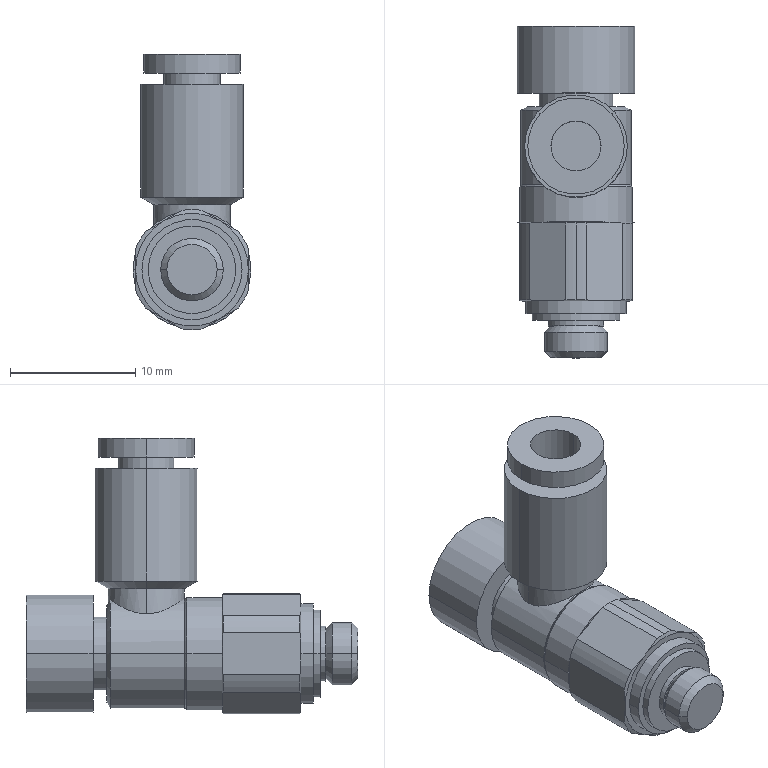Part | STEP file | speed control fitting AS1201F-M5-04SA | 1 solid | 77 faces | box 9.4 x 26.5 x 22 mm | volume 1970 mm3 | cylinder 34 | plane 25 | cone 18 | commonest cylinder face diameters 9.6 x7 8.8 x3 4 x2 4.4 x2 4.5 x2 5 x2